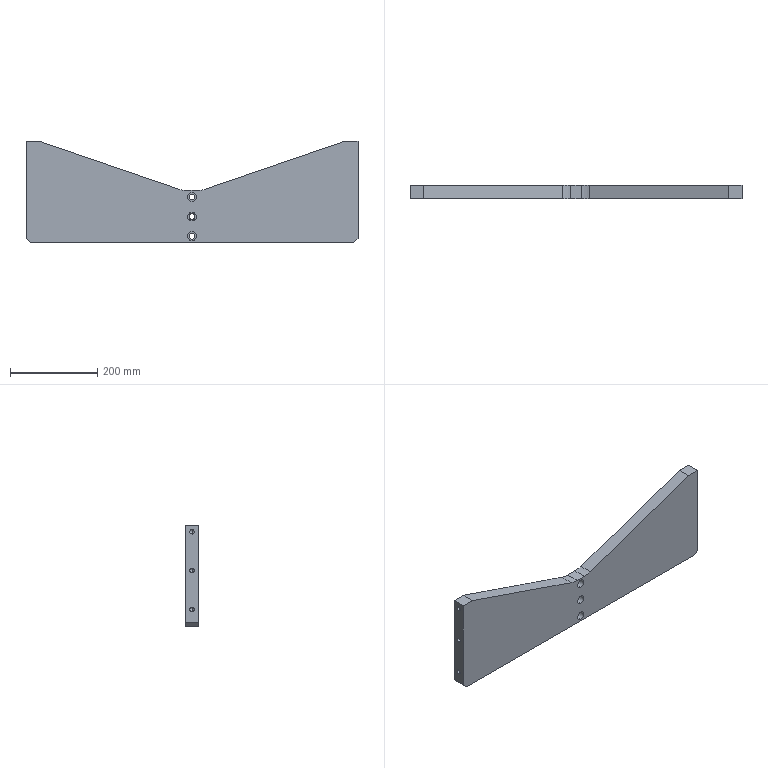Part | SolidWorks | features HoleWzd 4, Chamfer 1, Extrusion 1, Fillet 1, ICE 1 | 1 solid | 85 faces | box 763 x 30 x 233 mm | volume 4012044 mm3 | cylinder 42 | cone 28 | plane 15 | commonest cylinder face diameters 10.2 x28 13.5 x6 20 x6 120 x2